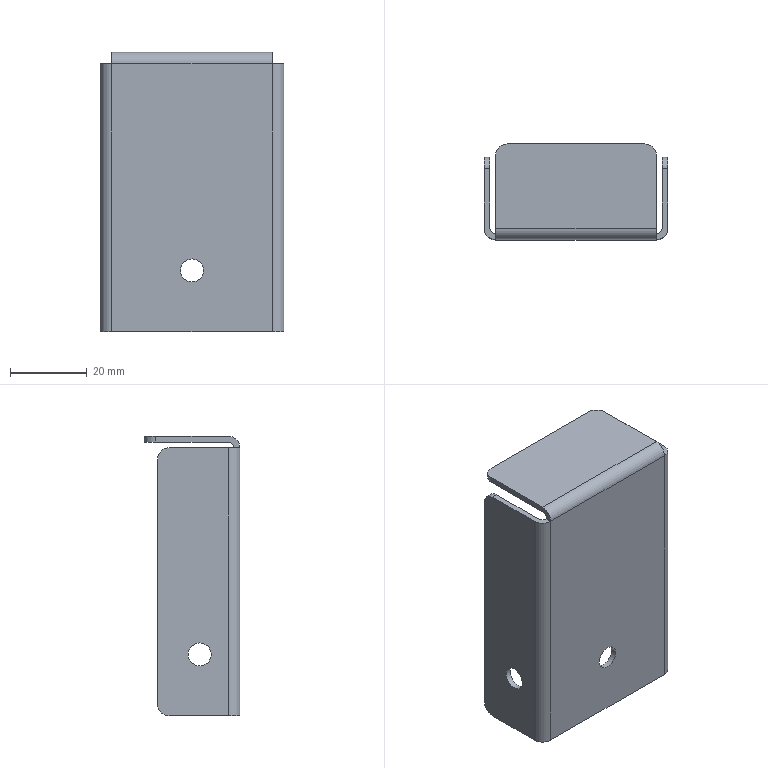Part | NX | features BREP 1 | 1 solid | 31 faces | box 48 x 25 x 73 mm | volume 10501 mm3 | plane 16 | cylinder 15 | commonest cylinder face diameters 6 x12 3 x3
STEP:
#1=CARTESIAN_POINT('',(1.5,0.,70.));
#2=VERTEX_POINT('',#1);
#3=CARTESIAN_POINT('',(43.5,0.,70.));
#4=VERTEX_POINT('',#3);
#5=CARTESIAN_POINT('',(0.,0.,70.));
#6=DIRECTION('',(1.,0.,0.));
#7=VECTOR('',#6,1000.);
#8=LINE('',#5,#7);
#9=EDGE_CURVE('',#2,#4,#8,.T.);
#10=ORIENTED_EDGE('',*,*,#9,.T.);
#11=CARTESIAN_POINT('',(43.5,0.,0.));
#12=VERTEX_POINT('',#11);
#13=CARTESIAN_POINT('',(43.5,0.,70.));
#14=DIRECTION('',(0.,0.,-1.));
#15=VECTOR('',#14,1000.);
#16=LINE('',#13,#15);
#17=EDGE_CURVE('',#4,#12,#16,.T.);
#18=ORIENTED_EDGE('',*,*,#17,.T.);
#19=CARTESIAN_POINT('',(1.5,0.,0.));
#20=VERTEX_POINT('',#19);
#21=CARTESIAN_POINT('',(0.,0.,0.));
#22=DIRECTION('',(-1.,0.,0.));
#23=VECTOR('',#22,1000.);
#24=LINE('',#21,#23);
#25=EDGE_CURVE('',#12,#20,#24,.T.);
#26=ORIENTED_EDGE('',*,*,#25,.T.);
#27=CARTESIAN_POINT('',(1.5,0.,70.));
#28=DIRECTION('',(0.,0.,1.));
#29=VECTOR('',#28,1000.);
#30=LINE('',#27,#29);
#31=EDGE_CURVE('',#20,#2,#30,.T.);
#32=ORIENTED_EDGE('',*,*,#31,.T.);
#33=EDGE_LOOP('',(#10,#18,#26,#32));
#34=FACE_BOUND('',#33,.T.);
#35=CARTESIAN_POINT('',(22.5,0.,19.));
#36=VERTEX_POINT('',#35);
#37=CARTESIAN_POINT('',(22.5,0.,16.));
#38=DIRECTION('',(0.,-1.,0.));
#39=DIRECTION('',(0.,0.,1.));
#40=AXIS2_PLACEMENT_3D('',#37,#38,#39);
#41=CIRCLE('',#40,3.);
#42=EDGE_CURVE('',#36,#36,#41,.T.);
#43=ORIENTED_EDGE('',*,*,#42,.T.);
#44=EDGE_LOOP('',(#43));
#45=FACE_BOUND('',#44,.T.);
#46=CARTESIAN_POINT('',(0.,0.,70.));
#47=DIRECTION('',(0.,1.,0.));
#48=DIRECTION('',(0.,0.,-1.));
#49=AXIS2_PLACEMENT_3D('',#46,#47,#48);
#50=PLANE('',#49);
#51=ADVANCED_FACE('',(#34,#45),#50,.T.);
#52=ORIENTED_EDGE('',*,*,#17,.F.);
#53=CARTESIAN_POINT('',(45.,1.5,70.));
#54=VERTEX_POINT('',#53);
#55=CARTESIAN_POINT('',(43.5,1.5,70.));
#56=DIRECTION('',(0.,0.,-1.));
#57=DIRECTION('',(-1.,0.,0.));
#58=AXIS2_PLACEMENT_3D('',#55,#56,#57);
#59=CIRCLE('',#58,1.5);
#60=EDGE_CURVE('',#54,#4,#59,.T.);
#61=ORIENTED_EDGE('',*,*,#60,.F.);
#62=CARTESIAN_POINT('',(45.,1.5,0.));
#63=VERTEX_POINT('',#62);
#64=CARTESIAN_POINT('',(45.,1.5,70.));
#65=DIRECTION('',(0.,0.,1.));
#66=VECTOR('',#65,1000.);
#67=LINE('',#64,#66);
#68=EDGE_CURVE('',#63,#54,#67,.T.);
#69=ORIENTED_EDGE('',*,*,#68,.F.);
#70=CARTESIAN_POINT('',(43.5,1.5,0.));
#71=DIRECTION('',(0.,0.,1.));
#72=DIRECTION('',(-1.,0.,0.));
#73=AXIS2_PLACEMENT_3D('',#70,#71,#72);
#74=CIRCLE('',#73,1.5);
#75=EDGE_CURVE('',#12,#63,#74,.T.);
#76=ORIENTED_EDGE('',*,*,#75,.F.);
#77=EDGE_LOOP('',(#52,#61,#69,#76));
#78=FACE_BOUND('',#77,.T.);
#79=CARTESIAN_POINT('',(43.5,1.5,70.));
#80=DIRECTION('',(0.,0.,-1.));
#81=DIRECTION('',(1.,0.,0.));
#82=AXIS2_PLACEMENT_3D('',#79,#80,#81);
#83=CYLINDRICAL_SURFACE('',#82,1.5);
#84=ADVANCED_FACE('',(#78),#83,.F.);
#85=CARTESIAN_POINT('',(1.5,1.5,71.5));
#86=VERTEX_POINT('',#85);
#87=CARTESIAN_POINT('',(1.5,1.5,70.));
#88=DIRECTION('',(1.,0.,0.));
#89=DIRECTION('',(0.,0.,-1.));
#90=AXIS2_PLACEMENT_3D('',#87,#88,#89);
#91=CIRCLE('',#90,1.5);
#92=EDGE_CURVE('',#86,#2,#91,.T.);
#93=ORIENTED_EDGE('',*,*,#92,.F.);
#94=CARTESIAN_POINT('',(43.5,1.5,71.5));
#95=VERTEX_POINT('',#94);
#96=CARTESIAN_POINT('',(43.5,1.5,71.5));
#97=DIRECTION('',(-1.,0.,0.));
#98=VECTOR('',#97,1000.);
#99=LINE('',#96,#98);
#100=EDGE_CURVE('',#95,#86,#99,.T.);
#101=ORIENTED_EDGE('',*,*,#100,.F.);
#102=CARTESIAN_POINT('',(43.5,1.5,70.));
#103=DIRECTION('',(-1.,0.,0.));
#104=DIRECTION('',(0.,0.,-1.));
#105=AXIS2_PLACEMENT_3D('',#102,#103,#104);
#106=CIRCLE('',#105,1.5);
#107=EDGE_CURVE('',#4,#95,#106,.T.);
#108=ORIENTED_EDGE('',*,*,#107,.F.);
#109=ORIENTED_EDGE('',*,*,#9,.F.);
#110=EDGE_LOOP('',(#93,#101,#108,#109));
#111=FACE_BOUND('',#110,.T.);
#112=CARTESIAN_POINT('',(43.5,1.5,70.));
#113=DIRECTION('',(1.,0.,0.));
#114=DIRECTION('',(0.,0.,1.));
#115=AXIS2_PLACEMENT_3D('',#112,#113,#114);
#116=CYLINDRICAL_SURFACE('',#115,1.5);
#117=ADVANCED_FACE('',(#111),#116,.F.);
#118=CARTESIAN_POINT('',(0.,1.5,70.));
#119=VERTEX_POINT('',#118);
#120=CARTESIAN_POINT('',(0.,1.5,0.));
#121=VERTEX_POINT('',#120);
#122=CARTESIAN_POINT('',(0.,1.5,70.));
#123=DIRECTION('',(0.,0.,-1.));
#124=VECTOR('',#123,1000.);
#125=LINE('',#122,#124);
#126=EDGE_CURVE('',#119,#121,#125,.T.);
#127=ORIENTED_EDGE('',*,*,#126,.F.);
#128=CARTESIAN_POINT('',(1.5,1.5,70.));
#129=DIRECTION('',(0.,0.,-1.));
#130=DIRECTION('',(-1.,0.,0.));
#131=AXIS2_PLACEMENT_3D('',#128,#129,#130);
#132=CIRCLE('',#131,1.5);
#133=EDGE_CURVE('',#2,#119,#132,.T.);
#134=ORIENTED_EDGE('',*,*,#133,.F.);
#135=ORIENTED_EDGE('',*,*,#31,.F.);
#136=CARTESIAN_POINT('',(1.5,1.5,0.));
#137=DIRECTION('',(0.,0.,1.));
#138=DIRECTION('',(-1.,0.,0.));
#139=AXIS2_PLACEMENT_3D('',#136,#137,#138);
#140=CIRCLE('',#139,1.5);
#141=EDGE_CURVE('',#121,#20,#140,.T.);
#142=ORIENTED_EDGE('',*,*,#141,.F.);
#143=EDGE_LOOP('',(#127,#134,#135,#142));
#144=FACE_BOUND('',#143,.T.);
#145=CARTESIAN_POINT('',(1.5,1.5,70.));
#146=DIRECTION('',(0.,0.,-1.));
#147=DIRECTION('',(1.,0.,0.));
#148=AXIS2_PLACEMENT_3D('',#145,#146,#147);
#149=CYLINDRICAL_SURFACE('',#148,1.5);
#150=ADVANCED_FACE('',(#144),#149,.F.);
#151=CARTESIAN_POINT('',(43.5,-1.5,0.));
#152=VERTEX_POINT('',#151);
#153=CARTESIAN_POINT('',(1.5,-1.5,0.));
#154=VERTEX_POINT('',#153);
#155=CARTESIAN_POINT('',(46.5,-1.5,0.));
#156=DIRECTION('',(-1.,0.,0.));
#157=VECTOR('',#156,1000.);
#158=LINE('',#155,#157);
#159=EDGE_CURVE('',#152,#154,#158,.T.);
#160=ORIENTED_EDGE('',*,*,#159,.T.);
#161=CARTESIAN_POINT('',(-1.5,1.5,0.));
#162=VERTEX_POINT('',#161);
#163=CARTESIAN_POINT('',(1.5,1.5,0.));
#164=DIRECTION('',(0.,0.,-1.));
#165=DIRECTION('',(-1.,0.,0.));
#166=AXIS2_PLACEMENT_3D('',#163,#164,#165);
#167=CIRCLE('',#166,3.);
#168=EDGE_CURVE('',#154,#162,#167,.T.);
#169=ORIENTED_EDGE('',*,*,#168,.T.);
#170=CARTESIAN_POINT('',(-1.5,17.,0.));
#171=VERTEX_POINT('',#170);
#172=CARTESIAN_POINT('',(-1.5,-1.5,0.));
#173=DIRECTION('',(0.,1.,0.));
#174=VECTOR('',#173,1000.);
#175=LINE('',#172,#174);
#176=EDGE_CURVE('',#162,#171,#175,.T.);
#177=ORIENTED_EDGE('',*,*,#176,.T.);
#178=CARTESIAN_POINT('',(0.,17.,0.));
#179=VERTEX_POINT('',#178);
#180=CARTESIAN_POINT('',(1.5,17.,0.));
#181=DIRECTION('',(-1.,0.,0.));
#182=VECTOR('',#181,1000.);
#183=LINE('',#180,#182);
#184=EDGE_CURVE('',#179,#171,#183,.T.);
#185=ORIENTED_EDGE('',*,*,#184,.F.);
#186=CARTESIAN_POINT('',(0.,20.,0.));
#187=DIRECTION('',(0.,1.,0.));
#188=VECTOR('',#187,1000.);
#189=LINE('',#186,#188);
#190=EDGE_CURVE('',#121,#179,#189,.T.);
#191=ORIENTED_EDGE('',*,*,#190,.F.);
#192=ORIENTED_EDGE('',*,*,#141,.T.);
#193=ORIENTED_EDGE('',*,*,#25,.F.);
#194=ORIENTED_EDGE('',*,*,#75,.T.);
#195=CARTESIAN_POINT('',(45.,17.,0.));
#196=VERTEX_POINT('',#195);
#197=CARTESIAN_POINT('',(45.,0.,0.));
#198=DIRECTION('',(0.,-1.,0.));
#199=VECTOR('',#198,1000.);
#200=LINE('',#197,#199);
#201=EDGE_CURVE('',#196,#63,#200,.T.);
#202=ORIENTED_EDGE('',*,*,#201,.F.);
#203=CARTESIAN_POINT('',(46.5,17.,0.));
#204=VERTEX_POINT('',#203);
#205=CARTESIAN_POINT('',(43.5,17.,0.));
#206=DIRECTION('',(1.,0.,0.));
#207=VECTOR('',#206,1000.);
#208=LINE('',#205,#207);
#209=EDGE_CURVE('',#196,#204,#208,.T.);
#210=ORIENTED_EDGE('',*,*,#209,.T.);
#211=CARTESIAN_POINT('',(46.5,1.5,0.));
#212=VERTEX_POINT('',#211);
#213=CARTESIAN_POINT('',(46.5,1.5,0.));
#214=DIRECTION('',(0.,-1.,0.));
#215=VECTOR('',#214,1000.);
#216=LINE('',#213,#215);
#217=EDGE_CURVE('',#204,#212,#216,.T.);
#218=ORIENTED_EDGE('',*,*,#217,.T.);
#219=CARTESIAN_POINT('',(43.5,1.5,0.));
#220=DIRECTION('',(0.,0.,-1.));
#221=DIRECTION('',(-1.,0.,0.));
#222=AXIS2_PLACEMENT_3D('',#219,#220,#221);
#223=CIRCLE('',#222,3.);
#224=EDGE_CURVE('',#212,#152,#223,.T.);
#225=ORIENTED_EDGE('',*,*,#224,.T.);
#226=EDGE_LOOP('',(#160,#169,#177,#185,#191,#192,#193,#194,#202,#210,#218,#225));
#227=FACE_BOUND('',#226,.T.);
#228=CARTESIAN_POINT('',(46.5,1.5,0.));
#229=DIRECTION('',(0.,0.,-1.));
#230=DIRECTION('',(1.,0.,0.));
#231=AXIS2_PLACEMENT_3D('',#228,#229,#230);
#232=PLANE('',#231);
#233=ADVANCED_FACE('',(#227),#232,.T.);
#234=ORIENTED_EDGE('',*,*,#42,.F.);
#235=EDGE_LOOP('',(#234));
#236=FACE_BOUND('',#235,.T.);
#237=CARTESIAN_POINT('',(22.5,-1.5,19.));
#238=VERTEX_POINT('',#237);
#239=CARTESIAN_POINT('',(22.5,-1.5,16.));
#240=DIRECTION('',(0.,1.,0.));
#241=DIRECTION('',(0.,0.,1.));
#242=AXIS2_PLACEMENT_3D('',#239,#240,#241);
#243=CIRCLE('',#242,3.);
#244=EDGE_CURVE('',#238,#238,#243,.T.);
#245=ORIENTED_EDGE('',*,*,#244,.F.);
#246=EDGE_LOOP('',(#245));
#247=FACE_BOUND('',#246,.T.);
#248=CARTESIAN_POINT('',(22.5,0.,16.));
#249=DIRECTION('',(0.,1.,0.));
#250=DIRECTION('',(0.,0.,-1.));
#251=AXIS2_PLACEMENT_3D('',#248,#249,#250);
#252=CYLINDRICAL_SURFACE('',#251,3.);
#253=ADVANCED_FACE('',(#236,#247),#252,.F.);
#254=CARTESIAN_POINT('',(43.5,-1.5,70.));
#255=VERTEX_POINT('',#254);
#256=CARTESIAN_POINT('',(43.5,1.5,70.));
#257=DIRECTION('',(0.,-1.,0.));
#258=VECTOR('',#257,1000.);
#259=LINE('',#256,#258);
#260=EDGE_CURVE('',#4,#255,#259,.T.);
#261=ORIENTED_EDGE('',*,*,#260,.T.);
#262=CARTESIAN_POINT('',(46.5,1.5,70.));
#263=VERTEX_POINT('',#262);
#264=CARTESIAN_POINT('',(43.5,1.5,70.));
#265=DIRECTION('',(0.,0.,1.));
#266=DIRECTION('',(-1.,0.,0.));
#267=AXIS2_PLACEMENT_3D('',#264,#265,#266);
#268=CIRCLE('',#267,3.);
#269=EDGE_CURVE('',#255,#263,#268,.T.);
#270=ORIENTED_EDGE('',*,*,#269,.T.);
#271=CARTESIAN_POINT('',(46.5,17.,70.));
#272=VERTEX_POINT('',#271);
#273=CARTESIAN_POINT('',(46.5,-1.5,70.));
#274=DIRECTION('',(0.,1.,0.));
#275=VECTOR('',#274,1000.);
#276=LINE('',#273,#275);
#277=EDGE_CURVE('',#263,#272,#276,.T.);
#278=ORIENTED_EDGE('',*,*,#277,.T.);
#279=CARTESIAN_POINT('',(45.,17.,70.));
#280=VERTEX_POINT('',#279);
#281=CARTESIAN_POINT('',(45.,17.,70.));
#282=DIRECTION('',(1.,0.,0.));
#283=VECTOR('',#282,1000.);
#284=LINE('',#281,#283);
#285=EDGE_CURVE('',#280,#272,#284,.T.);
#286=ORIENTED_EDGE('',*,*,#285,.F.);
#287=CARTESIAN_POINT('',(45.,0.,70.));
#288=DIRECTION('',(0.,1.,0.));
#289=VECTOR('',#288,1000.);
#290=LINE('',#287,#289);
#291=EDGE_CURVE('',#54,#280,#290,.T.);
#292=ORIENTED_EDGE('',*,*,#291,.F.);
#293=ORIENTED_EDGE('',*,*,#60,.T.);
#294=EDGE_LOOP('',(#261,#270,#278,#286,#292,#293));
#295=FACE_BOUND('',#294,.T.);
#296=CARTESIAN_POINT('',(45.,1.5,70.));
#297=DIRECTION('',(0.,0.,1.));
#298=DIRECTION('',(-1.,0.,0.));
#299=AXIS2_PLACEMENT_3D('',#296,#297,#298);
#300=PLANE('',#299);
#301=ADVANCED_FACE('',(#295),#300,.T.);
#302=ORIENTED_EDGE('',*,*,#201,.T.);
#303=ORIENTED_EDGE('',*,*,#68,.T.);
#304=ORIENTED_EDGE('',*,*,#291,.T.);
#305=CARTESIAN_POINT('',(45.,20.,67.));
#306=VERTEX_POINT('',#305);
#307=CARTESIAN_POINT('',(45.,17.,67.));
#308=DIRECTION('',(-1.,0.,0.));
#309=DIRECTION('',(0.,0.,-1.));
#310=AXIS2_PLACEMENT_3D('',#307,#308,#309);
#311=CIRCLE('',#310,3.);
#312=EDGE_CURVE('',#280,#306,#311,.T.);
#313=ORIENTED_EDGE('',*,*,#312,.T.);
#314=CARTESIAN_POINT('',(45.,20.,3.));
#315=VERTEX_POINT('',#314);
#316=CARTESIAN_POINT('',(45.,20.,70.));
#317=DIRECTION('',(0.,0.,-1.));
#318=VECTOR('',#317,1000.);
#319=LINE('',#316,#318);
#320=EDGE_CURVE('',#306,#315,#319,.T.);
#321=ORIENTED_EDGE('',*,*,#320,.T.);
#322=CARTESIAN_POINT('',(45.,17.,3.));
#323=DIRECTION('',(-1.,0.,0.));
#324=DIRECTION('',(0.,0.,-1.));
#325=AXIS2_PLACEMENT_3D('',#322,#323,#324);
#326=CIRCLE('',#325,3.);
#327=EDGE_CURVE('',#315,#196,#326,.T.);
#328=ORIENTED_EDGE('',*,*,#327,.T.);
#329=EDGE_LOOP('',(#302,#303,#304,#313,#321,#328));
#330=FACE_BOUND('',#329,.T.);
#331=CARTESIAN_POINT('',(45.,9.,19.));
#332=VERTEX_POINT('',#331);
#333=CARTESIAN_POINT('',(45.,9.,16.));
#334=DIRECTION('',(1.,0.,0.));
#335=DIRECTION('',(0.,0.,1.));
#336=AXIS2_PLACEMENT_3D('',#333,#334,#335);
#337=CIRCLE('',#336,3.);
#338=EDGE_CURVE('',#332,#332,#337,.T.);
#339=ORIENTED_EDGE('',*,*,#338,.T.);
#340=EDGE_LOOP('',(#339));
#341=FACE_BOUND('',#340,.T.);
#342=CARTESIAN_POINT('',(45.,0.,70.));
#343=DIRECTION('',(-1.,0.,0.));
#344=DIRECTION('',(0.,0.,-1.));
#345=AXIS2_PLACEMENT_3D('',#342,#343,#344);
#346=PLANE('',#345);
#347=ADVANCED_FACE('',(#330,#341),#346,.T.);
#348=CARTESIAN_POINT('',(1.5,-1.5,70.));
#349=VERTEX_POINT('',#348);
#350=CARTESIAN_POINT('',(1.5,1.5,70.));
#351=DIRECTION('',(0.,-1.,0.));
#352=VECTOR('',#351,1000.);
#353=LINE('',#350,#352);
#354=EDGE_CURVE('',#2,#349,#353,.T.);
#355=ORIENTED_EDGE('',*,*,#354,.T.);
#356=CARTESIAN_POINT('',(1.5,1.5,73.));
#357=VERTEX_POINT('',#356);
#358=CARTESIAN_POINT('',(1.5,1.5,70.));
#359=DIRECTION('',(-1.,0.,0.));
#360=DIRECTION('',(0.,0.,-1.));
#361=AXIS2_PLACEMENT_3D('',#358,#359,#360);
#362=CIRCLE('',#361,3.);
#363=EDGE_CURVE('',#349,#357,#362,.T.);
#364=ORIENTED_EDGE('',*,*,#363,.T.);
#365=CARTESIAN_POINT('',(1.5,20.5,73.));
#366=VERTEX_POINT('',#365);
#367=CARTESIAN_POINT('',(1.5,0.,73.));
#368=DIRECTION('',(0.,-1.,0.));
#369=VECTOR('',#368,1000.);
#370=LINE('',#367,#369);
#371=EDGE_CURVE('',#366,#357,#370,.T.);
#372=ORIENTED_EDGE('',*,*,#371,.F.);
#373=CARTESIAN_POINT('',(1.5,20.5,71.5));
#374=VERTEX_POINT('',#373);
#375=CARTESIAN_POINT('',(1.5,20.5,73.));
#376=DIRECTION('',(0.,0.,1.));
#377=VECTOR('',#376,1000.);
#378=LINE('',#375,#377);
#379=EDGE_CURVE('',#374,#366,#378,.T.);
#380=ORIENTED_EDGE('',*,*,#379,.F.);
#381=CARTESIAN_POINT('',(1.5,0.,71.5));
#382=DIRECTION('',(0.,1.,0.));
#383=VECTOR('',#382,1000.);
#384=LINE('',#381,#383);
#385=EDGE_CURVE('',#86,#374,#384,.T.);
#386=ORIENTED_EDGE('',*,*,#385,.F.);
#387=ORIENTED_EDGE('',*,*,#92,.T.);
#388=EDGE_LOOP('',(#355,#364,#372,#380,#386,#387));
#389=FACE_BOUND('',#388,.T.);
#390=CARTESIAN_POINT('',(1.5,1.5,70.));
#391=DIRECTION('',(-1.,0.,0.));
#392=DIRECTION('',(0.,0.,-1.));
#393=AXIS2_PLACEMENT_3D('',#390,#391,#392);
#394=PLANE('',#393);
#395=ADVANCED_FACE('',(#389),#394,.T.);
#396=CARTESIAN_POINT('',(43.5,20.5,71.5));
#397=VERTEX_POINT('',#396);
#398=CARTESIAN_POINT('',(43.5,0.,71.5));
#399=DIRECTION('',(0.,-1.,0.));
#400=VECTOR('',#399,1000.);
#401=LINE('',#398,#400);
#402=EDGE_CURVE('',#397,#95,#401,.T.);
#403=ORIENTED_EDGE('',*,*,#402,.T.);
#404=ORIENTED_EDGE('',*,*,#100,.T.);
#405=ORIENTED_EDGE('',*,*,#385,.T.);
#406=CARTESIAN_POINT('',(4.5,23.5,71.5));
#407=VERTEX_POINT('',#406);
#408=CARTESIAN_POINT('',(4.5,20.5,71.5));
#409=DIRECTION('',(0.,0.,-1.));
#410=DIRECTION('',(-1.,0.,0.));
#411=AXIS2_PLACEMENT_3D('',#408,#409,#410);
#412=CIRCLE('',#411,3.);
#413=EDGE_CURVE('',#374,#407,#412,.T.);
#414=ORIENTED_EDGE('',*,*,#413,.T.);
#415=CARTESIAN_POINT('',(40.5,23.5,71.5));
#416=VERTEX_POINT('',#415);
#417=CARTESIAN_POINT('',(0.,23.5,71.5));
#418=DIRECTION('',(1.,0.,0.));
#419=VECTOR('',#418,1000.);
#420=LINE('',#417,#419);
#421=EDGE_CURVE('',#407,#416,#420,.T.);
#422=ORIENTED_EDGE('',*,*,#421,.T.);
#423=CARTESIAN_POINT('',(40.5,20.5,71.5));
#424=DIRECTION('',(0.,0.,-1.));
#425=DIRECTION('',(-1.,0.,0.));
#426=AXIS2_PLACEMENT_3D('',#423,#424,#425);
#427=CIRCLE('',#426,3.);
#428=EDGE_CURVE('',#416,#397,#427,.T.);
#429=ORIENTED_EDGE('',*,*,#428,.T.);
#430=EDGE_LOOP('',(#403,#404,#405,#414,#422,#429));
#431=FACE_BOUND('',#430,.T.);
#432=CARTESIAN_POINT('',(0.,0.,71.5));
#433=DIRECTION('',(0.,0.,-1.));
#434=DIRECTION('',(1.,0.,0.));
#435=AXIS2_PLACEMENT_3D('',#432,#433,#434);
#436=PLANE('',#435);
#437=ADVANCED_FACE('',(#431),#436,.T.);
#438=ORIENTED_EDGE('',*,*,#107,.T.);
#439=ORIENTED_EDGE('',*,*,#402,.F.);
#440=CARTESIAN_POINT('',(43.5,20.5,73.));
#441=VERTEX_POINT('',#440);
#442=CARTESIAN_POINT('',(43.5,20.5,73.));
#443=DIRECTION('',(0.,0.,-1.));
#444=VECTOR('',#443,1000.);
#445=LINE('',#442,#444);
#446=EDGE_CURVE('',#441,#397,#445,.T.);
#447=ORIENTED_EDGE('',*,*,#446,.F.);
#448=CARTESIAN_POINT('',(43.5,1.5,73.));
#449=VERTEX_POINT('',#448);
#450=CARTESIAN_POINT('',(43.5,23.5,73.));
#451=DIRECTION('',(0.,1.,0.));
#452=VECTOR('',#451,1000.);
#453=LINE('',#450,#452);
#454=EDGE_CURVE('',#449,#441,#453,.T.);
#455=ORIENTED_EDGE('',*,*,#454,.F.);
#456=CARTESIAN_POINT('',(43.5,1.5,70.));
#457=DIRECTION('',(-1.,0.,0.));
#458=DIRECTION('',(0.,0.,-1.));
#459=AXIS2_PLACEMENT_3D('',#456,#457,#458);
#460=CIRCLE('',#459,3.);
#461=EDGE_CURVE('',#255,#449,#460,.T.);
#462=ORIENTED_EDGE('',*,*,#461,.F.);
#463=ORIENTED_EDGE('',*,*,#260,.F.);
#464=EDGE_LOOP('',(#438,#439,#447,#455,#462,#463));
#465=FACE_BOUND('',#464,.T.);
#466=CARTESIAN_POINT('',(43.5,1.5,70.));
#467=DIRECTION('',(-1.,0.,0.));
#468=DIRECTION('',(0.,0.,-1.));
#469=AXIS2_PLACEMENT_3D('',#466,#467,#468);
#470=PLANE('',#469);
#471=ADVANCED_FACE('',(#465),#470,.F.);
#472=ORIENTED_EDGE('',*,*,#190,.T.);
#473=CARTESIAN_POINT('',(0.,20.,3.));
#474=VERTEX_POINT('',#473);
#475=CARTESIAN_POINT('',(0.,17.,3.));
#476=DIRECTION('',(1.,0.,0.));
#477=DIRECTION('',(0.,0.,-1.));
#478=AXIS2_PLACEMENT_3D('',#475,#476,#477);
#479=CIRCLE('',#478,3.);
#480=EDGE_CURVE('',#179,#474,#479,.T.);
#481=ORIENTED_EDGE('',*,*,#480,.T.);
#482=CARTESIAN_POINT('',(0.,20.,67.));
#483=VERTEX_POINT('',#482);
#484=CARTESIAN_POINT('',(0.,20.,70.));
#485=DIRECTION('',(0.,0.,1.));
#486=VECTOR('',#485,1000.);
#487=LINE('',#484,#486);
#488=EDGE_CURVE('',#474,#483,#487,.T.);
#489=ORIENTED_EDGE('',*,*,#488,.T.);
#490=CARTESIAN_POINT('',(0.,17.,70.));
#491=VERTEX_POINT('',#490);
#492=CARTESIAN_POINT('',(0.,17.,67.));
#493=DIRECTION('',(1.,0.,0.));
#494=DIRECTION('',(0.,0.,1.));
#495=AXIS2_PLACEMENT_3D('',#492,#493,#494);
#496=CIRCLE('',#495,3.);
#497=EDGE_CURVE('',#483,#491,#496,.T.);
#498=ORIENTED_EDGE('',*,*,#497,.T.);
#499=CARTESIAN_POINT('',(0.,20.,70.));
#500=DIRECTION('',(0.,-1.,0.));
#501=VECTOR('',#500,1000.);
#502=LINE('',#499,#501);
#503=EDGE_CURVE('',#491,#119,#502,.T.);
#504=ORIENTED_EDGE('',*,*,#503,.T.);
#505=ORIENTED_EDGE('',*,*,#126,.T.);
#506=EDGE_LOOP('',(#472,#481,#489,#498,#504,#505));
#507=FACE_BOUND('',#506,.T.);
#508=CARTESIAN_POINT('',(0.,9.,13.));
#509=VERTEX_POINT('',#508);
#510=CARTESIAN_POINT('',(0.,9.,16.));
#511=DIRECTION('',(-1.,0.,0.));
#512=DIRECTION('',(0.,0.,-1.));
#513=AXIS2_PLACEMENT_3D('',#510,#511,#512);
#514=CIRCLE('',#513,3.);
#515=EDGE_CURVE('',#509,#509,#514,.T.);
#516=ORIENTED_EDGE('',*,*,#515,.T.);
#517=EDGE_LOOP('',(#516));
#518=FACE_BOUND('',#517,.T.);
#519=CARTESIAN_POINT('',(0.,20.,70.));
#520=DIRECTION('',(1.,0.,0.));
#521=DIRECTION('',(0.,-1.,0.));
#522=AXIS2_PLACEMENT_3D('',#519,#520,#521);
#523=PLANE('',#522);
#524=ADVANCED_FACE('',(#507,#518),#523,.T.);
#525=ORIENTED_EDGE('',*,*,#133,.T.);
#526=ORIENTED_EDGE('',*,*,#503,.F.);
#527=CARTESIAN_POINT('',(-1.5,17.,70.));
#528=VERTEX_POINT('',#527);
#529=CARTESIAN_POINT('',(43.5,17.,70.));
#530=DIRECTION('',(1.,0.,0.));
#531=VECTOR('',#530,1000.);
#532=LINE('',#529,#531);
#533=EDGE_CURVE('',#528,#491,#532,.T.);
#534=ORIENTED_EDGE('',*,*,#533,.F.);
#535=CARTESIAN_POINT('',(-1.5,1.5,70.));
#536=VERTEX_POINT('',#535);
#537=CARTESIAN_POINT('',(-1.5,1.5,70.));
#538=DIRECTION('',(0.,1.,0.));
#539=VECTOR('',#538,1000.);
#540=LINE('',#537,#539);
#541=EDGE_CURVE('',#536,#528,#540,.T.);
#542=ORIENTED_EDGE('',*,*,#541,.F.);
#543=CARTESIAN_POINT('',(1.5,1.5,70.));
#544=DIRECTION('',(0.,0.,1.));
#545=DIRECTION('',(-1.,0.,0.));
#546=AXIS2_PLACEMENT_3D('',#543,#544,#545);
#547=CIRCLE('',#546,3.);
#548=EDGE_CURVE('',#536,#349,#547,.T.);
#549=ORIENTED_EDGE('',*,*,#548,.T.);
#550=ORIENTED_EDGE('',*,*,#354,.F.);
#551=EDGE_LOOP('',(#525,#526,#534,#542,#549,#550));
#552=FACE_BOUND('',#551,.T.);
#553=CARTESIAN_POINT('',(1.5,0.,70.));
#554=DIRECTION('',(0.,0.,1.));
#555=DIRECTION('',(-1.,0.,0.));
#556=AXIS2_PLACEMENT_3D('',#553,#554,#555);
#557=PLANE('',#556);
#558=ADVANCED_FACE('',(#552),#557,.T.);
#559=CARTESIAN_POINT('',(43.5,-1.5,70.));
#560=DIRECTION('',(0.,0.,-1.));
#561=VECTOR('',#560,1000.);
#562=LINE('',#559,#561);
#563=EDGE_CURVE('',#255,#152,#562,.T.);
#564=ORIENTED_EDGE('',*,*,#563,.F.);
#565=CARTESIAN_POINT('',(0.,-1.5,70.));
#566=DIRECTION('',(1.,0.,0.));
#567=VECTOR('',#566,1000.);
#568=LINE('',#565,#567);
#569=EDGE_CURVE('',#349,#255,#568,.T.);
#570=ORIENTED_EDGE('',*,*,#569,.F.);
#571=CARTESIAN_POINT('',(1.5,-1.5,70.));
#572=DIRECTION('',(0.,0.,1.));
#573=VECTOR('',#572,1000.);
#574=LINE('',#571,#573);
#575=EDGE_CURVE('',#154,#349,#574,.T.);
#576=ORIENTED_EDGE('',*,*,#575,.F.);
#577=ORIENTED_EDGE('',*,*,#159,.F.);
#578=EDGE_LOOP('',(#564,#570,#576,#577));
#579=FACE_BOUND('',#578,.T.);
#580=ORIENTED_EDGE('',*,*,#244,.T.);
#581=EDGE_LOOP('',(#580));
#582=FACE_BOUND('',#581,.T.);
#583=CARTESIAN_POINT('',(0.,-1.5,70.));
#584=DIRECTION('',(0.,1.,0.));
#585=DIRECTION('',(0.,0.,-1.));
#586=AXIS2_PLACEMENT_3D('',#583,#584,#585);
#587=PLANE('',#586);
#588=ADVANCED_FACE('',(#579,#582),#587,.F.);
#589=ORIENTED_EDGE('',*,*,#269,.F.);
#590=ORIENTED_EDGE('',*,*,#563,.T.);
#591=ORIENTED_EDGE('',*,*,#224,.F.);
#592=CARTESIAN_POINT('',(46.5,1.5,70.));
#593=DIRECTION('',(0.,0.,1.));
#594=VECTOR('',#593,1000.);
#595=LINE('',#592,#594);
#596=EDGE_CURVE('',#212,#263,#595,.T.);
#597=ORIENTED_EDGE('',*,*,#596,.T.);
#598=EDGE_LOOP('',(#589,#590,#591,#597));
#599=FACE_BOUND('',#598,.T.);
#600=CARTESIAN_POINT('',(43.5,1.5,70.));
#601=DIRECTION('',(0.,0.,-1.));
#602=DIRECTION('',(1.,0.,0.));
#603=AXIS2_PLACEMENT_3D('',#600,#601,#602);
#604=CYLINDRICAL_SURFACE('',#603,3.);
#605=ADVANCED_FACE('',(#599),#604,.T.);
#606=CARTESIAN_POINT('',(46.5,20.,3.));
#607=VERTEX_POINT('',#606);
#608=CARTESIAN_POINT('',(46.5,17.,3.));
#609=DIRECTION('',(-1.,0.,0.));
#610=DIRECTION('',(0.,0.,-1.));
#611=AXIS2_PLACEMENT_3D('',#608,#609,#610);
#612=CIRCLE('',#611,3.);
#613=EDGE_CURVE('',#607,#204,#612,.T.);
#614=ORIENTED_EDGE('',*,*,#613,.T.);
#615=ORIENTED_EDGE('',*,*,#209,.F.);
#616=ORIENTED_EDGE('',*,*,#327,.F.);
#617=CARTESIAN_POINT('',(43.5,20.,3.));
#618=DIRECTION('',(1.,0.,0.));
#619=VECTOR('',#618,1000.);
#620=LINE('',#617,#619);
#621=EDGE_CURVE('',#315,#607,#620,.T.);
#622=ORIENTED_EDGE('',*,*,#621,.T.);
#623=EDGE_LOOP('',(#614,#615,#616,#622));
#624=FACE_BOUND('',#623,.T.);
#625=CARTESIAN_POINT('',(43.5,17.,3.));
#626=DIRECTION('',(1.,0.,0.));
#627=DIRECTION('',(0.,0.,1.));
#628=AXIS2_PLACEMENT_3D('',#625,#626,#627);
#629=CYLINDRICAL_SURFACE('',#628,3.);
#630=ADVANCED_FACE('',(#624),#629,.T.);
#631=CARTESIAN_POINT('',(46.5,20.,67.));
#632=VERTEX_POINT('',#631);
#633=CARTESIAN_POINT('',(46.5,20.,70.));
#634=DIRECTION('',(0.,0.,-1.));
#635=VECTOR('',#634,1000.);
#636=LINE('',#633,#635);
#637=EDGE_CURVE('',#632,#607,#636,.T.);
#638=ORIENTED_EDGE('',*,*,#637,.T.);
#639=ORIENTED_EDGE('',*,*,#621,.F.);
#640=ORIENTED_EDGE('',*,*,#320,.F.);
#641=CARTESIAN_POINT('',(45.,20.,67.));
#642=DIRECTION('',(1.,0.,0.));
#643=VECTOR('',#642,1000.);
#644=LINE('',#641,#643);
#645=EDGE_CURVE('',#306,#632,#644,.T.);
#646=ORIENTED_EDGE('',*,*,#645,.T.);
#647=EDGE_LOOP('',(#638,#639,#640,#646));
#648=FACE_BOUND('',#647,.T.);
#649=CARTESIAN_POINT('',(45.,20.,70.));
#650=DIRECTION('',(0.,1.,0.));
#651=DIRECTION('',(0.,0.,-1.));
#652=AXIS2_PLACEMENT_3D('',#649,#650,#651);
#653=PLANE('',#652);
#654=ADVANCED_FACE('',(#648),#653,.T.);
#655=CARTESIAN_POINT('',(46.5,17.,67.));
#656=DIRECTION('',(-1.,0.,0.));
#657=DIRECTION('',(0.,0.,-1.));
#658=AXIS2_PLACEMENT_3D('',#655,#656,#657);
#659=CIRCLE('',#658,3.);
#660=EDGE_CURVE('',#272,#632,#659,.T.);
#661=ORIENTED_EDGE('',*,*,#660,.T.);
#662=ORIENTED_EDGE('',*,*,#645,.F.);
#663=ORIENTED_EDGE('',*,*,#312,.F.);
#664=ORIENTED_EDGE('',*,*,#285,.T.);
#665=EDGE_LOOP('',(#661,#662,#663,#664));
#666=FACE_BOUND('',#665,.T.);
#667=CARTESIAN_POINT('',(45.,17.,67.));
#668=DIRECTION('',(1.,0.,0.));
#669=DIRECTION('',(0.,0.,1.));
#670=AXIS2_PLACEMENT_3D('',#667,#668,#669);
#671=CYLINDRICAL_SURFACE('',#670,3.);
#672=ADVANCED_FACE('',(#666),#671,.T.);
#673=ORIENTED_EDGE('',*,*,#338,.F.);
#674=EDGE_LOOP('',(#673));
#675=FACE_BOUND('',#674,.T.);
#676=CARTESIAN_POINT('',(46.5,9.,19.));
#677=VERTEX_POINT('',#676);
#678=CARTESIAN_POINT('',(46.5,9.,16.));
#679=DIRECTION('',(-1.,0.,0.));
#680=DIRECTION('',(0.,0.,1.));
#681=AXIS2_PLACEMENT_3D('',#678,#679,#680);
#682=CIRCLE('',#681,3.);
#683=EDGE_CURVE('',#677,#677,#682,.T.);
#684=ORIENTED_EDGE('',*,*,#683,.F.);
#685=EDGE_LOOP('',(#684));
#686=FACE_BOUND('',#685,.T.);
#687=CARTESIAN_POINT('',(45.,9.,16.));
#688=DIRECTION('',(-1.,0.,0.));
#689=DIRECTION('',(0.,0.,-1.));
#690=AXIS2_PLACEMENT_3D('',#687,#688,#689);
#691=CYLINDRICAL_SURFACE('',#690,3.);
#692=ADVANCED_FACE('',(#675,#686),#691,.F.);
#693=CARTESIAN_POINT('',(43.5,1.5,73.));
#694=DIRECTION('',(-1.,0.,0.));
#695=VECTOR('',#694,1000.);
#696=LINE('',#693,#695);
#697=EDGE_CURVE('',#449,#357,#696,.T.);
#698=ORIENTED_EDGE('',*,*,#697,.T.);
#699=ORIENTED_EDGE('',*,*,#363,.F.);
#700=ORIENTED_EDGE('',*,*,#569,.T.);
#701=ORIENTED_EDGE('',*,*,#461,.T.);
#702=EDGE_LOOP('',(#698,#699,#700,#701));
#703=FACE_BOUND('',#702,.T.);
#704=CARTESIAN_POINT('',(43.5,1.5,70.));
#705=DIRECTION('',(1.,0.,0.));
#706=DIRECTION('',(0.,0.,1.));
#707=AXIS2_PLACEMENT_3D('',#704,#705,#706);
#708=CYLINDRICAL_SURFACE('',#707,3.);
#709=ADVANCED_FACE('',(#703),#708,.T.);
#710=ORIENTED_EDGE('',*,*,#428,.F.);
#711=CARTESIAN_POINT('',(40.5,23.5,73.));
#712=VERTEX_POINT('',#711);
#713=CARTESIAN_POINT('',(40.5,23.5,73.));
#714=DIRECTION('',(0.,0.,1.));
#715=VECTOR('',#714,1000.);
#716=LINE('',#713,#715);
#717=EDGE_CURVE('',#416,#712,#716,.T.);
#718=ORIENTED_EDGE('',*,*,#717,.T.);
#719=CARTESIAN_POINT('',(40.5,20.5,73.));
#720=DIRECTION('',(0.,0.,-1.));
#721=DIRECTION('',(-1.,0.,0.));
#722=AXIS2_PLACEMENT_3D('',#719,#720,#721);
#723=CIRCLE('',#722,3.);
#724=EDGE_CURVE('',#712,#441,#723,.T.);
#725=ORIENTED_EDGE('',*,*,#724,.T.);
#726=ORIENTED_EDGE('',*,*,#446,.T.);
#727=EDGE_LOOP('',(#710,#718,#725,#726));
#728=FACE_BOUND('',#727,.T.);
#729=CARTESIAN_POINT('',(40.5,20.5,73.));
#730=DIRECTION('',(0.,0.,-1.));
#731=DIRECTION('',(1.,0.,0.));
#732=AXIS2_PLACEMENT_3D('',#729,#730,#731);
#733=CYLINDRICAL_SURFACE('',#732,3.);
#734=ADVANCED_FACE('',(#728),#733,.T.);
#735=CARTESIAN_POINT('',(4.5,23.5,73.));
#736=VERTEX_POINT('',#735);
#737=CARTESIAN_POINT('',(4.5,23.5,73.));
#738=DIRECTION('',(0.,0.,-1.));
#739=VECTOR('',#738,1000.);
#740=LINE('',#737,#739);
#741=EDGE_CURVE('',#736,#407,#740,.T.);
#742=ORIENTED_EDGE('',*,*,#741,.F.);
#743=CARTESIAN_POINT('',(1.5,23.5,73.));
#744=DIRECTION('',(-1.,0.,0.));
#745=VECTOR('',#744,1000.);
#746=LINE('',#743,#745);
#747=EDGE_CURVE('',#712,#736,#746,.T.);
#748=ORIENTED_EDGE('',*,*,#747,.F.);
#749=ORIENTED_EDGE('',*,*,#717,.F.);
#750=ORIENTED_EDGE('',*,*,#421,.F.);
#751=EDGE_LOOP('',(#742,#748,#749,#750));
#752=FACE_BOUND('',#751,.T.);
#753=CARTESIAN_POINT('',(1.5,23.5,73.));
#754=DIRECTION('',(0.,-1.,0.));
#755=DIRECTION('',(0.,0.,1.));
#756=AXIS2_PLACEMENT_3D('',#753,#754,#755);
#757=PLANE('',#756);
#758=ADVANCED_FACE('',(#752),#757,.F.);
#759=ORIENTED_EDGE('',*,*,#413,.F.);
#760=ORIENTED_EDGE('',*,*,#379,.T.);
#761=CARTESIAN_POINT('',(4.5,20.5,73.));
#762=DIRECTION('',(0.,0.,-1.));
#763=DIRECTION('',(-1.,0.,0.));
#764=AXIS2_PLACEMENT_3D('',#761,#762,#763);
#765=CIRCLE('',#764,3.);
#766=EDGE_CURVE('',#366,#736,#765,.T.);
#767=ORIENTED_EDGE('',*,*,#766,.T.);
#768=ORIENTED_EDGE('',*,*,#741,.T.);
#769=EDGE_LOOP('',(#759,#760,#767,#768));
#770=FACE_BOUND('',#769,.T.);
#771=CARTESIAN_POINT('',(4.5,20.5,73.));
#772=DIRECTION('',(0.,0.,-1.));
#773=DIRECTION('',(1.,0.,0.));
#774=AXIS2_PLACEMENT_3D('',#771,#772,#773);
#775=CYLINDRICAL_SURFACE('',#774,3.);
#776=ADVANCED_FACE('',(#770),#775,.T.);
#777=ORIENTED_EDGE('',*,*,#548,.F.);
#778=CARTESIAN_POINT('',(-1.5,1.5,70.));
#779=DIRECTION('',(0.,0.,-1.));
#780=VECTOR('',#779,1000.);
#781=LINE('',#778,#780);
#782=EDGE_CURVE('',#536,#162,#781,.T.);
#783=ORIENTED_EDGE('',*,*,#782,.T.);
#784=ORIENTED_EDGE('',*,*,#168,.F.);
#785=ORIENTED_EDGE('',*,*,#575,.T.);
#786=EDGE_LOOP('',(#777,#783,#784,#785));
#787=FACE_BOUND('',#786,.T.);
#788=CARTESIAN_POINT('',(1.5,1.5,70.));
#789=DIRECTION('',(0.,0.,-1.));
#790=DIRECTION('',(1.,0.,0.));
#791=AXIS2_PLACEMENT_3D('',#788,#789,#790);
#792=CYLINDRICAL_SURFACE('',#791,3.);
#793=ADVANCED_FACE('',(#787),#792,.T.);
#794=ORIENTED_EDGE('',*,*,#480,.F.);
#795=ORIENTED_EDGE('',*,*,#184,.T.);
#796=CARTESIAN_POINT('',(-1.5,20.,3.));
#797=VERTEX_POINT('',#796);
#798=CARTESIAN_POINT('',(-1.5,17.,3.));
#799=DIRECTION('',(1.,0.,0.));
#800=DIRECTION('',(0.,0.,-1.));
#801=AXIS2_PLACEMENT_3D('',#798,#799,#800);
#802=CIRCLE('',#801,3.);
#803=EDGE_CURVE('',#171,#797,#802,.T.);
#804=ORIENTED_EDGE('',*,*,#803,.T.);
#805=CARTESIAN_POINT('',(1.5,20.,3.));
#806=DIRECTION('',(1.,0.,0.));
#807=VECTOR('',#806,1000.);
#808=LINE('',#805,#807);
#809=EDGE_CURVE('',#797,#474,#808,.T.);
#810=ORIENTED_EDGE('',*,*,#809,.T.);
#811=EDGE_LOOP('',(#794,#795,#804,#810));
#812=FACE_BOUND('',#811,.T.);
#813=CARTESIAN_POINT('',(1.5,17.,3.));
#814=DIRECTION('',(1.,0.,0.));
#815=DIRECTION('',(0.,0.,1.));
#816=AXIS2_PLACEMENT_3D('',#813,#814,#815);
#817=CYLINDRICAL_SURFACE('',#816,3.);
#818=ADVANCED_FACE('',(#812),#817,.T.);
#819=ORIENTED_EDGE('',*,*,#497,.F.);
#820=CARTESIAN_POINT('',(-1.5,20.,67.));
#821=VERTEX_POINT('',#820);
#822=CARTESIAN_POINT('',(-1.5,20.,67.));
#823=DIRECTION('',(-1.,0.,0.));
#824=VECTOR('',#823,1000.);
#825=LINE('',#822,#824);
#826=EDGE_CURVE('',#483,#821,#825,.T.);
#827=ORIENTED_EDGE('',*,*,#826,.T.);
#828=CARTESIAN_POINT('',(-1.5,17.,67.));
#829=DIRECTION('',(1.,0.,0.));
#830=DIRECTION('',(0.,0.,1.));
#831=AXIS2_PLACEMENT_3D('',#828,#829,#830);
#832=CIRCLE('',#831,3.);
#833=EDGE_CURVE('',#821,#528,#832,.T.);
#834=ORIENTED_EDGE('',*,*,#833,.T.);
#835=ORIENTED_EDGE('',*,*,#533,.T.);
#836=EDGE_LOOP('',(#819,#827,#834,#835));
#837=FACE_BOUND('',#836,.T.);
#838=CARTESIAN_POINT('',(-1.5,17.,67.));
#839=DIRECTION('',(-1.,0.,0.));
#840=DIRECTION('',(0.,0.,-1.));
#841=AXIS2_PLACEMENT_3D('',#838,#839,#840);
#842=CYLINDRICAL_SURFACE('',#841,3.);
#843=ADVANCED_FACE('',(#837),#842,.T.);
#844=ORIENTED_EDGE('',*,*,#488,.F.);
#845=ORIENTED_EDGE('',*,*,#809,.F.);
#846=CARTESIAN_POINT('',(-1.5,20.,70.));
#847=DIRECTION('',(0.,0.,1.));
#848=VECTOR('',#847,1000.);
#849=LINE('',#846,#848);
#850=EDGE_CURVE('',#797,#821,#849,.T.);
#851=ORIENTED_EDGE('',*,*,#850,.T.);
#852=ORIENTED_EDGE('',*,*,#826,.F.);
#853=EDGE_LOOP('',(#844,#845,#851,#852));
#854=FACE_BOUND('',#853,.T.);
#855=CARTESIAN_POINT('',(-1.5,20.,70.));
#856=DIRECTION('',(0.,1.,0.));
#857=DIRECTION('',(0.,0.,-1.));
#858=AXIS2_PLACEMENT_3D('',#855,#856,#857);
#859=PLANE('',#858);
#860=ADVANCED_FACE('',(#854),#859,.T.);
#861=ORIENTED_EDGE('',*,*,#515,.F.);
#862=EDGE_LOOP('',(#861));
#863=FACE_BOUND('',#862,.T.);
#864=CARTESIAN_POINT('',(-1.5,9.,13.));
#865=VERTEX_POINT('',#864);
#866=CARTESIAN_POINT('',(-1.5,9.,16.));
#867=DIRECTION('',(1.,0.,0.));
#868=DIRECTION('',(0.,0.,-1.));
#869=AXIS2_PLACEMENT_3D('',#866,#867,#868);
#870=CIRCLE('',#869,3.);
#871=EDGE_CURVE('',#865,#865,#870,.T.);
#872=ORIENTED_EDGE('',*,*,#871,.F.);
#873=EDGE_LOOP('',(#872));
#874=FACE_BOUND('',#873,.T.);
#875=CARTESIAN_POINT('',(0.,9.,16.));
#876=DIRECTION('',(1.,0.,0.));
#877=DIRECTION('',(0.,0.,1.));
#878=AXIS2_PLACEMENT_3D('',#875,#876,#877);
#879=CYLINDRICAL_SURFACE('',#878,3.);
#880=ADVANCED_FACE('',(#863,#874),#879,.F.);
#881=ORIENTED_EDGE('',*,*,#660,.F.);
#882=ORIENTED_EDGE('',*,*,#277,.F.);
#883=ORIENTED_EDGE('',*,*,#596,.F.);
#884=ORIENTED_EDGE('',*,*,#217,.F.);
#885=ORIENTED_EDGE('',*,*,#613,.F.);
#886=ORIENTED_EDGE('',*,*,#637,.F.);
#887=EDGE_LOOP('',(#881,#882,#883,#884,#885,#886));
#888=FACE_BOUND('',#887,.T.);
#889=ORIENTED_EDGE('',*,*,#683,.T.);
#890=EDGE_LOOP('',(#889));
#891=FACE_BOUND('',#890,.T.);
#892=CARTESIAN_POINT('',(46.5,0.,70.));
#893=DIRECTION('',(-1.,0.,0.));
#894=DIRECTION('',(0.,0.,-1.));
#895=AXIS2_PLACEMENT_3D('',#892,#893,#894);
#896=PLANE('',#895);
#897=ADVANCED_FACE('',(#888,#891),#896,.F.);
#898=ORIENTED_EDGE('',*,*,#766,.F.);
#899=ORIENTED_EDGE('',*,*,#371,.T.);
#900=ORIENTED_EDGE('',*,*,#697,.F.);
#901=ORIENTED_EDGE('',*,*,#454,.T.);
#902=ORIENTED_EDGE('',*,*,#724,.F.);
#903=ORIENTED_EDGE('',*,*,#747,.T.);
#904=EDGE_LOOP('',(#898,#899,#900,#901,#902,#903));
#905=FACE_BOUND('',#904,.T.);
#906=CARTESIAN_POINT('',(0.,0.,73.));
#907=DIRECTION('',(0.,0.,-1.));
#908=DIRECTION('',(1.,0.,0.));
#909=AXIS2_PLACEMENT_3D('',#906,#907,#908);
#910=PLANE('',#909);
#911=ADVANCED_FACE('',(#905),#910,.F.);
#912=ORIENTED_EDGE('',*,*,#833,.F.);
#913=ORIENTED_EDGE('',*,*,#850,.F.);
#914=ORIENTED_EDGE('',*,*,#803,.F.);
#915=ORIENTED_EDGE('',*,*,#176,.F.);
#916=ORIENTED_EDGE('',*,*,#782,.F.);
#917=ORIENTED_EDGE('',*,*,#541,.T.);
#918=EDGE_LOOP('',(#912,#913,#914,#915,#916,#917));
#919=FACE_BOUND('',#918,.T.);
#920=ORIENTED_EDGE('',*,*,#871,.T.);
#921=EDGE_LOOP('',(#920));
#922=FACE_BOUND('',#921,.T.);
#923=CARTESIAN_POINT('',(-1.5,20.,70.));
#924=DIRECTION('',(1.,0.,0.));
#925=DIRECTION('',(0.,-1.,0.));
#926=AXIS2_PLACEMENT_3D('',#923,#924,#925);
#927=PLANE('',#926);
#928=ADVANCED_FACE('',(#919,#922),#927,.F.);
#929=CLOSED_SHELL('',(#51,#84,#117,#150,#233,#253,#301,#347,#395,#437,#471,#524,#558,#588,#605,#630,#654,#672,#692,#709,#734,#758,#776,#793,#818,#843,#860,#880,#897,#911,#928));
#930=MANIFOLD_SOLID_BREP('',#929);
#931=(LENGTH_UNIT()NAMED_UNIT(*)SI_UNIT(.MILLI.,.METRE.));
#932=UNCERTAINTY_MEASURE_WITH_UNIT(LENGTH_MEASURE(0.00001),#931,'','');
#933=(NAMED_UNIT(*)PLANE_ANGLE_UNIT()SI_UNIT($,.RADIAN.));
#934=(NAMED_UNIT(*)SI_UNIT($,.STERADIAN.)SOLID_ANGLE_UNIT());
#935=(GEOMETRIC_REPRESENTATION_CONTEXT(3)GLOBAL_UNCERTAINTY_ASSIGNED_CONTEXT((#932))GLOBAL_UNIT_ASSIGNED_CONTEXT((#931,#933,#934))REPRESENTATION_CONTEXT('',''));
#936=ADVANCED_BREP_SHAPE_REPRESENTATION('',(#930),#935);